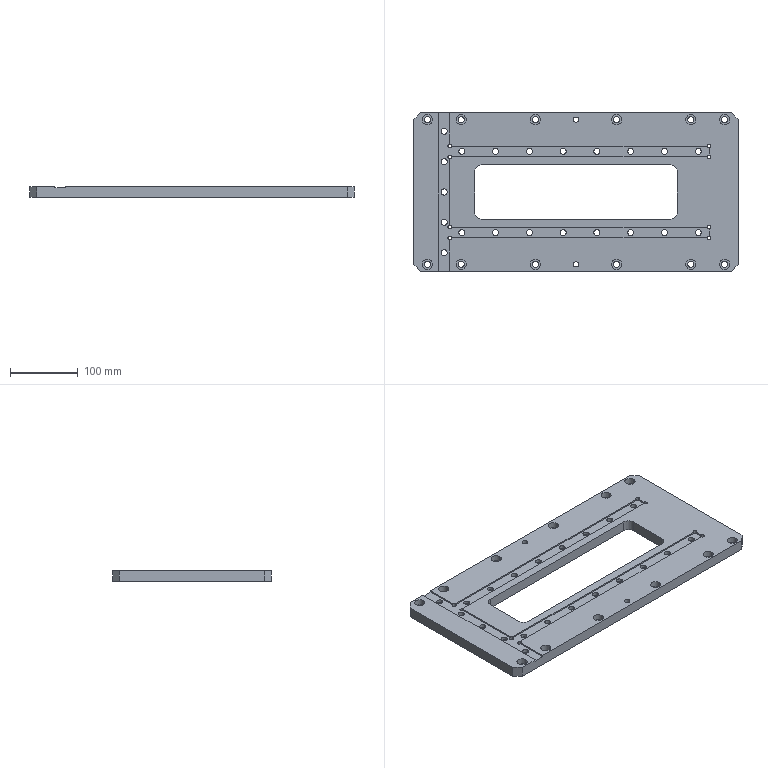Part | SolidWorks | features HoleWzd 5, ICE 3, Chamfer 1, Extrusion 1, Fillet 1, LPattern 1 | 1 solid | 215 faces | box 480 x 235 x 16 mm | volume 1317910 mm3 | cylinder 156 | plane 59 | commonest cylinder face diameters 9 x66 15 x66 5.5 x16 8 x4 20 x4